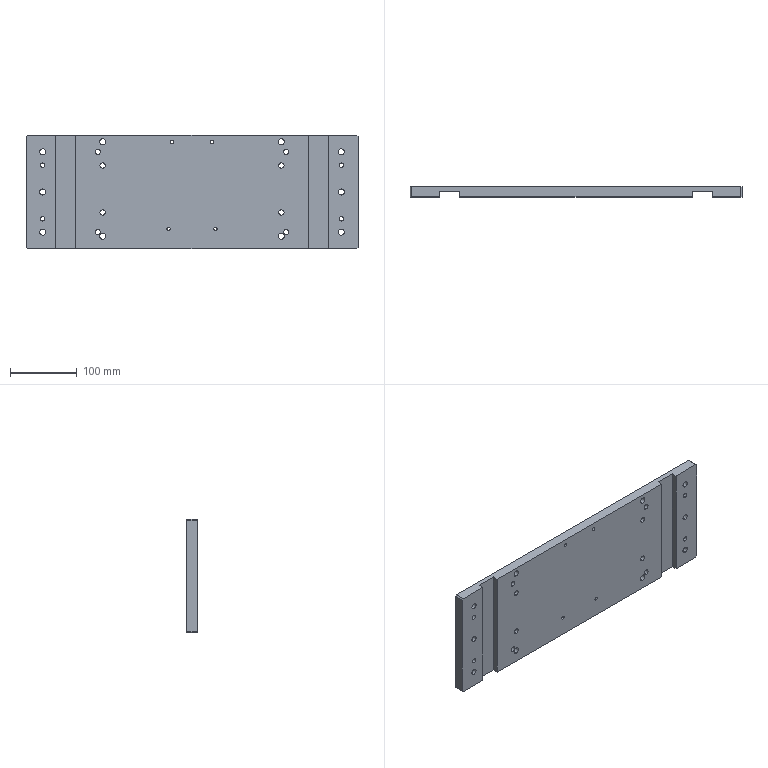Part | SolidWorks | features HoleWzd 7, ICE 2, Chamfer 1, Cut 1, Extrusion 1, MirrorPattern 1 | 1 solid | 122 faces | box 496 x 15 x 170 mm | volume 1153313 mm3 | cylinder 84 | plane 28 | cone 10 | commonest cylinder face diameters 15 x22 9 x20 5 x18 8 x16 6.8 x8